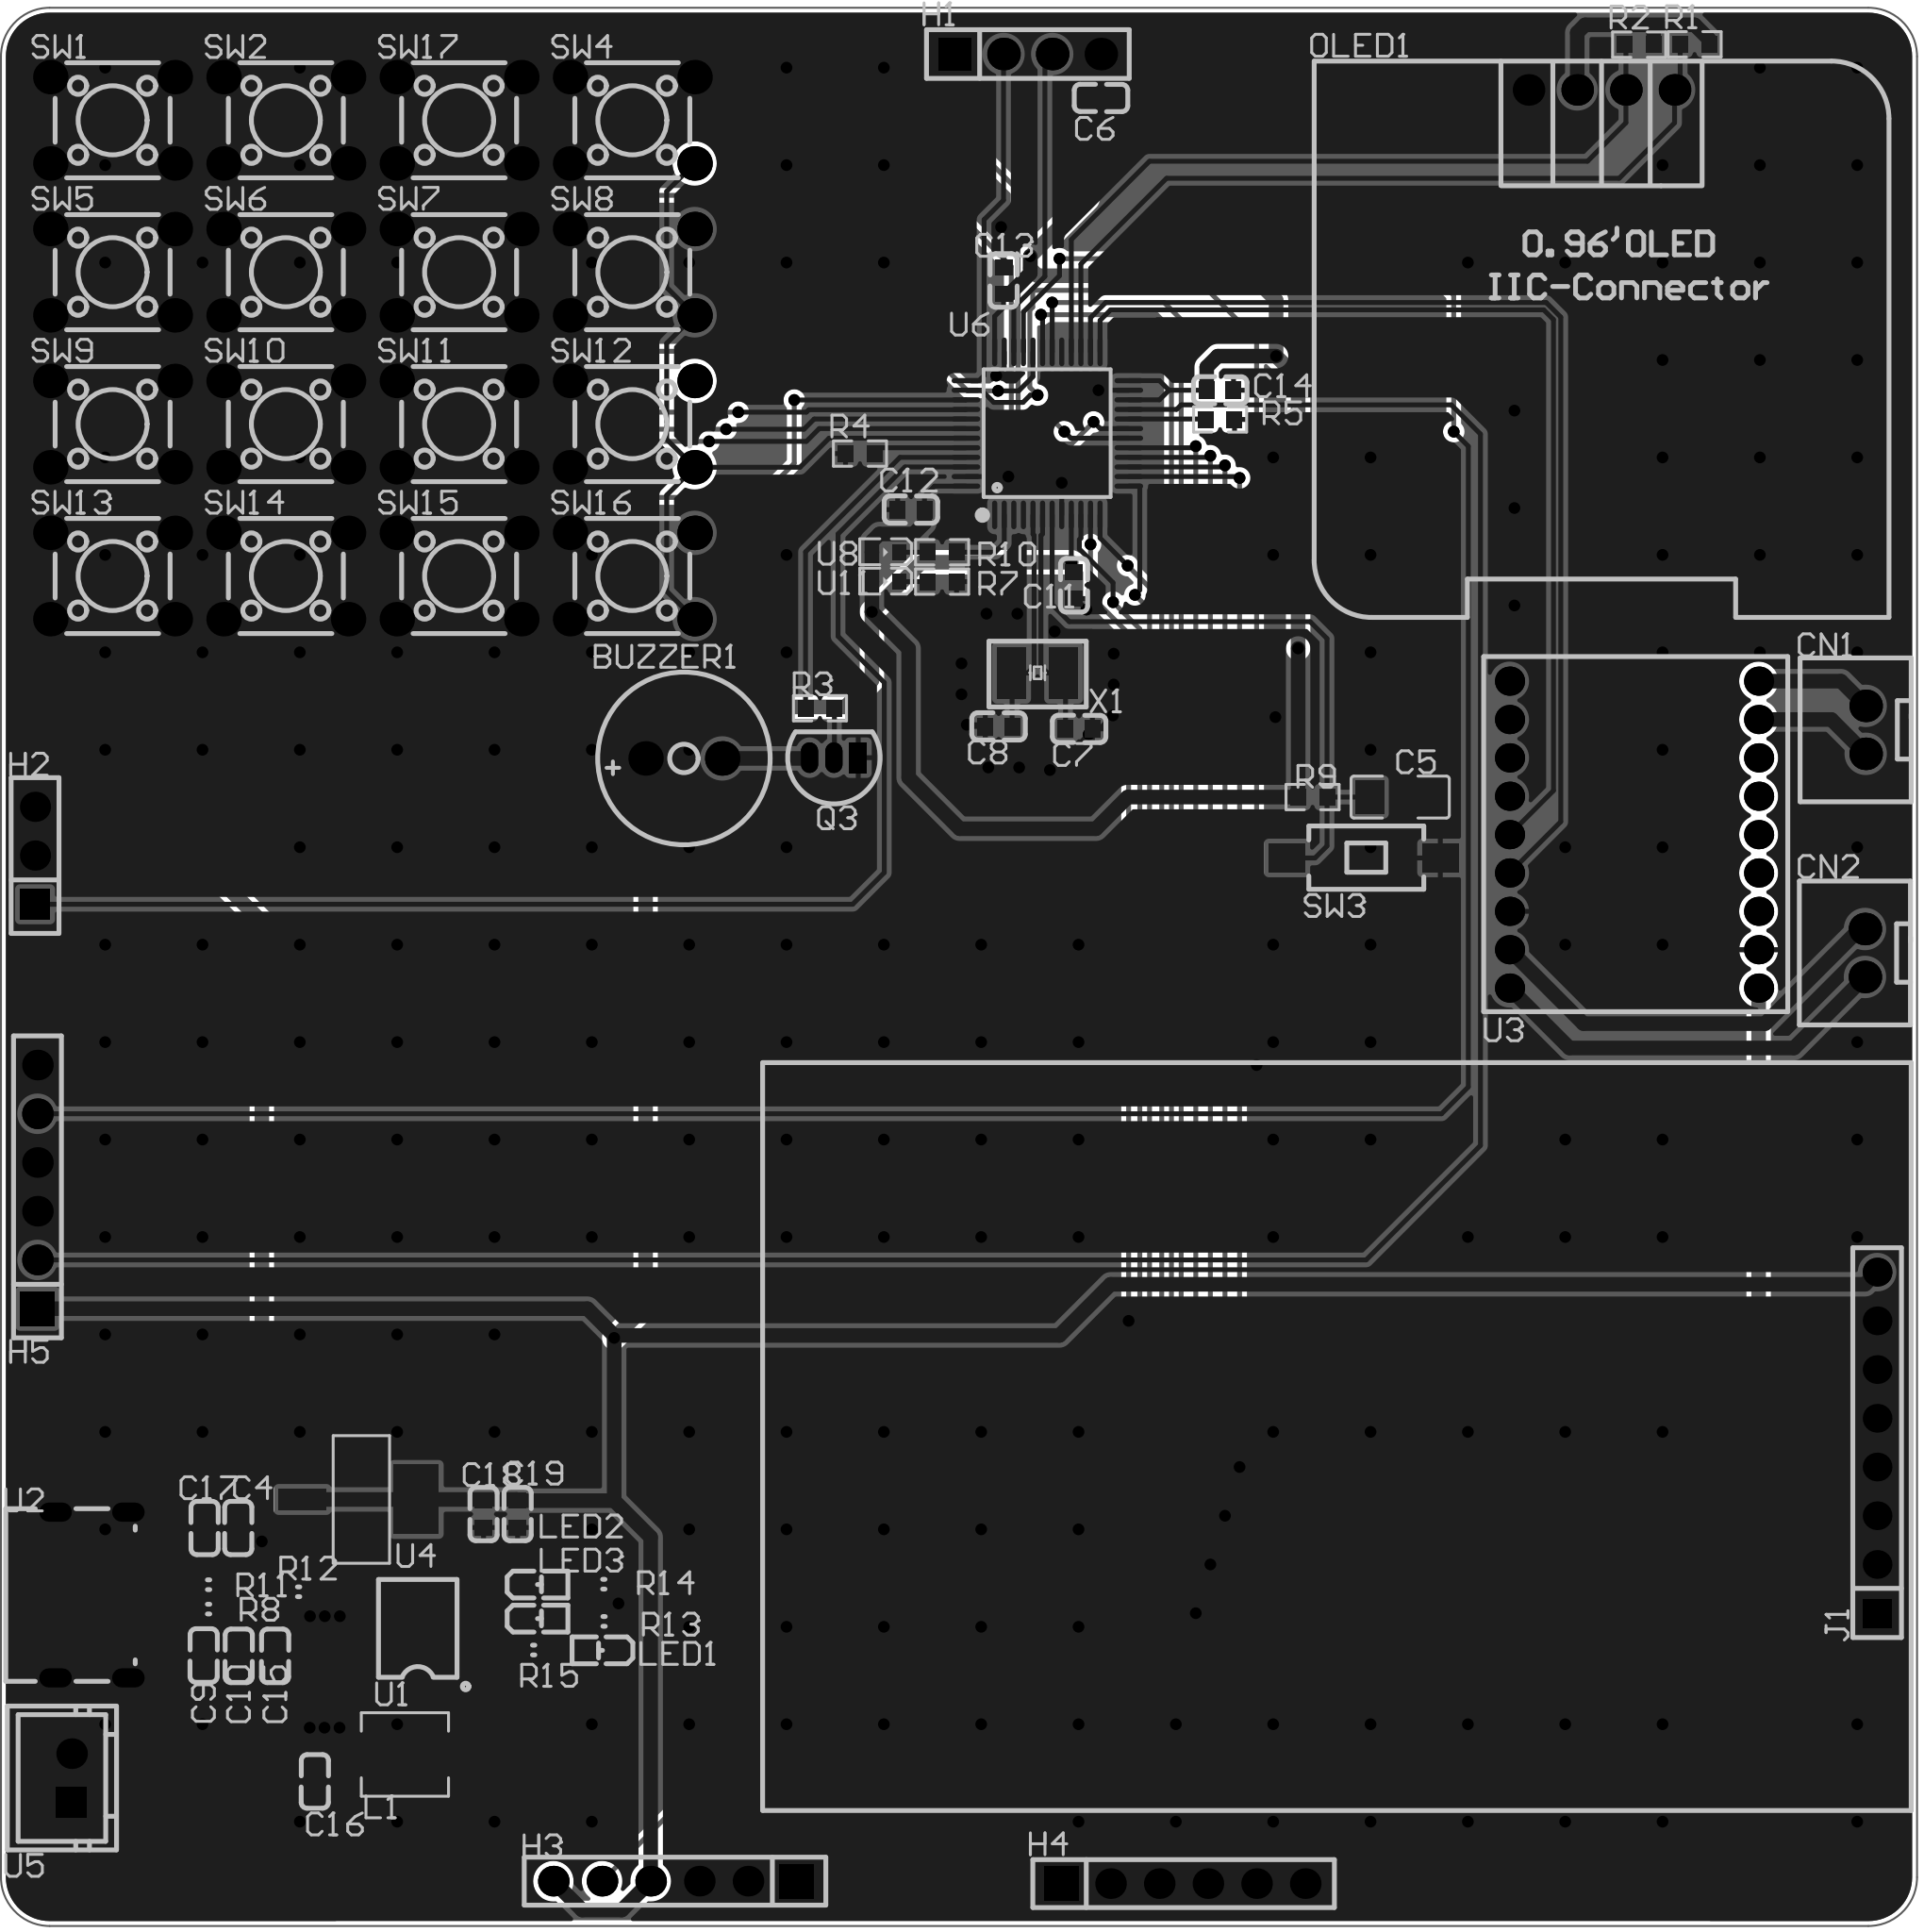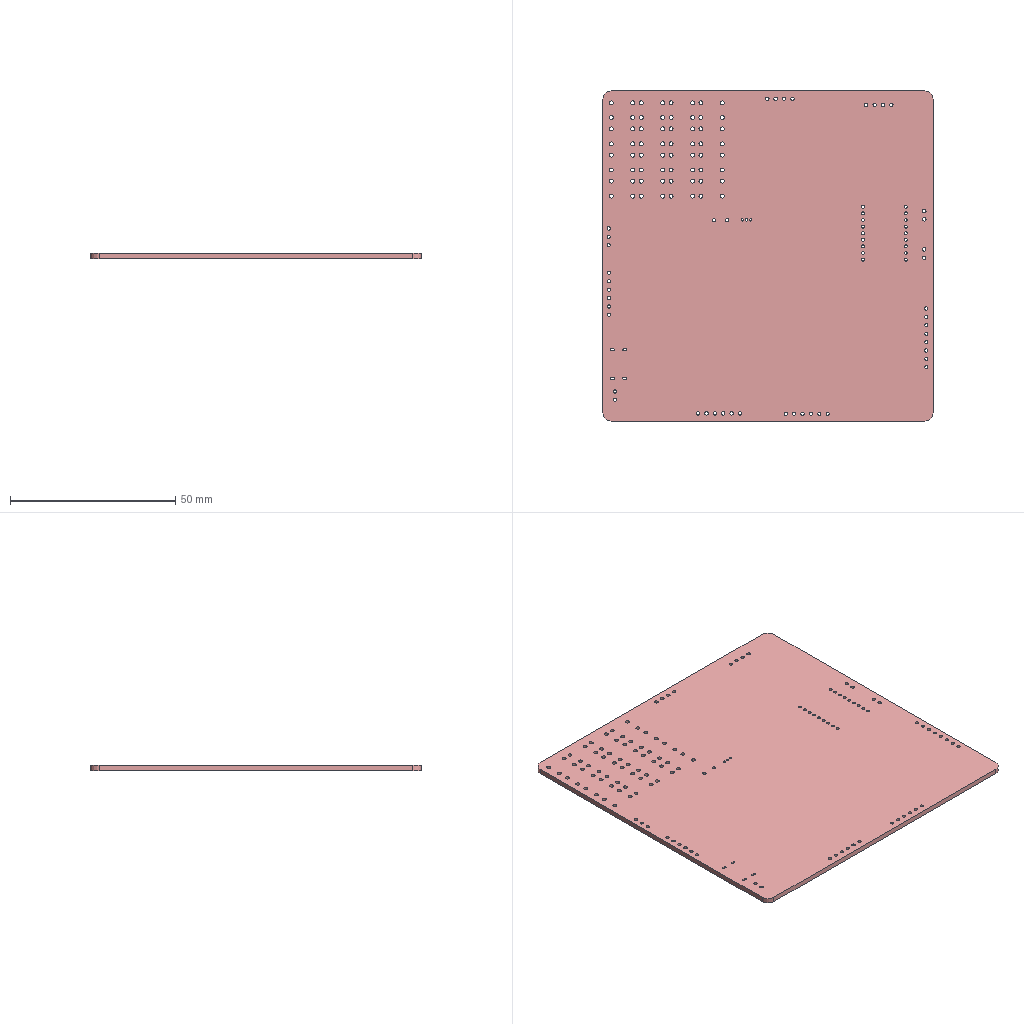Circuit board layout | Altium Designer | box 100 x 100 x 1.6 mm
Layer stack:
# Altium Designer layer stack of  (unit mm; dielectric type: 0 none, 1 core, 2 prepreg, 3 surface material)
index,name,kind,layer,copper_thickness_mm,dielectric_type,dielectric_thickness_mm,dielectric_material,dielectric_constant
0,Top Paste Mask Layer,other,,,,,,
1,Top Silkscreen Layer,other,,,,,,
2,Top Solder Mask Layer,dielectric,,,3,0.01,,3.3
3,Top Layer,copper,Top Layer,0.035,,,,
4,Dielectric1,dielectric,,,3,1.51,FR4,4.5
5,Bottom Layer,copper,Bottom Layer,0.035,,,,
6,Bottom Solder Mask Layer,dielectric,,,3,0.01,,3.3
7,Bottom Silkscreen Layer,other,,,,,,
8,Bottom Paste Mask Layer,other,,,,,,
# drill layer pairs: low layer,high layer
drill_pair,Top Layer,Bottom Layer
Part placement:
Designator,Comment,Layer,Footprint,Center-X(mm),Center-Y(mm),Rotation
BUZZER1,2.7kHz,TopLayer,BUZ-TH_BD9.0-P4.00-D0.6-FD,115.399,144.382,0
C4,10uF,TopLayer,C0603,92.139,104.263,270
C5,100uF,TopLayer,C1206,152.781,142.367,180
C6,100nF,TopLayer,C0603,137.16,178.816,180
C7,20pF,TopLayer,C0603,136.017,145.923,180
C8,20pF,TopLayer,C0603,131.826,146.05,0
C9,22uF,TopLayer,C0603,90.337,97.623,90
C10,22uF,TopLayer,C0603,92.167,97.605,90
C11,100nF,TopLayer,C0603,135.763,153.416,90
C12,100nF,TopLayer,C0603,127.254,157.353,0
C13,100nF,TopLayer,C0603,132.08,169.291,270
C14,100nF,TopLayer,C0603,143.383,163.576,180
C15,22uF,TopLayer,C0603,94.066,97.605,90
C16,22uF,TopLayer,C0603,96.139,91.059,90
C17,100nF,TopLayer,C0603,90.383,104.263,270
C18,10uF,TopLayer,C0603,104.942,104.989,90
C19,100nF,TopLayer,C0603,106.72,104.989,90
CN1,XH2.54*2P_直插,TopLayer,CONN-TH_2P-P2.50-XH2.54-2P,177.077,145.871,270
CN2,XH2.54*2P_直插,TopLayer,CONN-TH_2P-P2.50-XH2.54-2P,177.038,134.239,270
H1,,TopLayer,HDR-TH_4P-P2.54-V-F,133.35,181.102,0
H2,,TopLayer,HDR-TH_3P-P2.54-V-F,81.534,139.319,90
H3,,TopLayer,HDR-TH_6P-P2.54-V-F,114.935,85.852,180
H4,,TopLayer,HDR-TH_6P-P2.54-V-F,141.478,85.725,0
H5,,TopLayer,HDR-TH_6P-P2.54-V-F,81.661,122.047,90
J1,,TopLayer,HDR-TH_8P-P2.54-V-M,177.673,108.712,90
L1,2.2uH,TopLayer,IND-SMD_L4.4-W4.2,100.838,92.456,180
LED1,电池,TopLayer,LED0603_L1.6-W0.8-RD_BLUE,111.033,97.885,180
LED2,放电,TopLayer,LED0603_L1.6-W0.8-RD_BLUE,107.874,101.316,0
LED3,充电,TopLayer,LED0603_L1.6-W0.8-RD_BLUE,107.874,99.538,0
OLED1,,TopLayer,0.96OLED_4P,163.291,179.234,0
Q3,,TopLayer,S8050_TO_92,123.226,144.422,180
R1,5.1K,TopLayer,R0603,168.148,181.61,0
R2,5.1K,TopLayer,R0603,165.252,181.593,0
R4,10kΩ,TopLayer,R0603,124.587,160.274,0
R5,10kΩ,TopLayer,R0603,143.383,162.052,180
R7,510Ω,TopLayer,R0603,128.875,153.599,0
R8,5.1K,TopLayer,R0603-NSK,90.591,100.036,180
R9,1kΩ,TopLayer,R0603,148.209,142.367,180
R10,510Ω,TopLayer,R0603,128.875,155.131,0
R11,5.1K,TopLayer,R0603-NSK,90.591,101.306,180
R12,56K,TopLayer,R0603-NSK,95.29,100.937,180
R13,5.1K,TopLayer,R0603-NSK,111.232,99.394,180
R14,5.1K,TopLayer,R0603-NSK,111.218,101.333,180
R15,5.1K,TopLayer,R0603-NSK,107.557,97.901,180
SW1,KH-6X6X6H-TJ,TopLayer,SW-TH_4P-L6.0-W6.0-P4.50-LS6.5,85.583,177.649,0
SW2,KH-6X6X6H-TJ,TopLayer,SW-TH_4P-L6.0-W6.0-P4.50-LS6.5,94.624,177.649,0
SW3,TS-1101-C-W,TopLayer,SW-SMD_L6.0-W3.3-LS8.0,150.876,139.192,180
SW4,KH-6X6X6H-TJ,TopLayer,SW-TH_4P-L6.0-W6.0-P4.50-LS6.5,112.707,177.649,0
SW5,KH-6X6X6H-TJ,TopLayer,SW-TH_4P-L6.0-W6.0-P4.50-LS6.5,85.583,169.73,0
SW6,KH-6X6X6H-TJ,TopLayer,SW-TH_4P-L6.0-W6.0-P4.50-LS6.5,94.624,169.73,0
SW7,KH-6X6X6H-TJ,TopLayer,SW-TH_4P-L6.0-W6.0-P4.50-LS6.5,103.666,169.73,0
SW8,KH-6X6X6H-TJ,TopLayer,SW-TH_4P-L6.0-W6.0-P4.50-LS6.5,112.707,169.73,0
SW9,KH-6X6X6H-TJ,TopLayer,SW-TH_4P-L6.0-W6.0-P4.50-LS6.5,85.583,161.81,0
SW10,KH-6X6X6H-TJ,TopLayer,SW-TH_4P-L6.0-W6.0-P4.50-LS6.5,94.624,161.81,0
SW11,KH-6X6X6H-TJ,TopLayer,SW-TH_4P-L6.0-W6.0-P4.50-LS6.5,103.666,161.81,0
SW12,KH-6X6X6H-TJ,TopLayer,SW-TH_4P-L6.0-W6.0-P4.50-LS6.5,112.707,161.81,0
SW13,KH-6X6X6H-TJ,TopLayer,SW-TH_4P-L6.0-W6.0-P4.50-LS6.5,85.583,153.892,0
SW14,KH-6X6X6H-TJ,TopLayer,SW-TH_4P-L6.0-W6.0-P4.50-LS6.5,94.624,153.892,0
SW15,KH-6X6X6H-TJ,TopLayer,SW-TH_4P-L6.0-W6.0-P4.50-LS6.5,103.666,153.892,0
SW16,KH-6X6X6H-TJ,TopLayer,SW-TH_4P-L6.0-W6.0-P4.50-LS6.5,112.707,153.892,0
SW17,KH-6X6X6H-TJ,TopLayer,SW-TH_4P-L6.0-W6.0-P4.50-LS6.5,103.666,177.649,0
U1,ETA9742,TopLayer,ESOP-8_L4.9-W3.9-P1.27-LS6.0-BL-EP,101.508,99.03,90
U2,YTC-TC6-268,TopLayer,TYPE-C-SMD_YIYUAN_YTC-TC6-268,84.731,100.77,270
U3,CON2.0MM-PAD-18,TopLayer,CONN-TH_18P-P2.00_C9900078766,164.989,140.41,90
U4,AMS1117-3.3,TopLayer,SOT-223-3_L6.5-W3.4-P2.30-LS7.0-BR,98.465,105.751,180
U6,STM32F103C8T6,TopLayer,LQFP-48_L7.0-W7.0-P0.50-LS9.0-BL,134.367,161.326,0
U8,42-51/GHC-YW2X2K/3T,TopLayer,LED-SMD_L1.6-W0.8-FD_GREEN-1,125.925,155.131,0
U11,42-51/GHC-YW2X2K/3T,TopLayer,LED-SMD_L1.6-W0.8-FD_GREEN-1,125.925,153.599,0
X1,8MHz,TopLayer,CRYSTAL-SMD_L3.2-W2.5_3225-8MHZ,133.858,148.844,180
R3,1K,TopLayer,R0603,122.501,146.998,180
U5,_x001F_XH2.54-2P,TopLayer,CONN-TH_2P-P2.54-V,83.445,91.23,90
Pad and via stacks:
# Altium Designer via and pad stacks of  (unit mm). Each distinct definition once, with the count of objects using it.
# via: kind,start_layer,end_layer,hole_mm,diameter_mm,mode(0 simple;1 top-mid-bottom;2 full stack),diameter_per_layer,count,example_net
# pad: kind,layer,hole_mm,hole_type(0 round;1 square;2 slot),plating,top_size,top_shape(1 round;2 rect;3 octagon;9 rounded rect),mid_size,bottom_size,mode,footprint,size_per_layer,count,example
pad,Multi-Layer,1,0,plated,1.8x1.8,1,1.8x1.8,1.8x1.8,0,BUZ-TH_BD9.0-P4.00-D0.6-FD,,2,BUZZER1.1
pad,Multi-Layer,1.05,0,plated,1.7x1.7,1,1.7x1.7,1.7x1.7,0,CONN-TH_2P-P2.50-XH2.54-2P,,4,CN1.2
pad,Multi-Layer,1.1,0,plated,1.7x1.7,2,1.7x1.7,1.7x1.7,0,HDR-TH_4P-P2.54-V-F,,1,H1.1
pad,Multi-Layer,1.1,0,plated,1.7x1.7,1,1.7x1.7,1.7x1.7,0,HDR-TH_4P-P2.54-V-F,,3,H1.2
pad,Multi-Layer,1.02,0,plated,1.575x1.575,1,1.575x1.575,1.575x1.575,0,HDR-TH_3P-P2.54-V-F,,2,H2.3
pad,Multi-Layer,1.02,0,plated,1.575x1.575,2,1.575x1.575,1.575x1.575,0,HDR-TH_3P-P2.54-V-F,,1,H2.1
pad,Multi-Layer,1.02,0,plated,1.6x1.6,1,1.6x1.6,1.6x1.6,0,HDR-TH_6P-P2.54-V-F,,15,H3.6
pad,Multi-Layer,1.02,0,plated,1.8x1.8,2,1.8x1.8,1.8x1.8,0,HDR-TH_6P-P2.54-V-F,,3,H3.1
pad,Multi-Layer,1,0,plated,1.5x1.5,2,1.5x1.5,1.5x1.5,0,HDR-TH_8P-P2.54-V-M,,1,J1.1
pad,Multi-Layer,1,0,plated,1.5x1.5,1,1.5x1.5,1.5x1.5,0,HDR-TH_8P-P2.54-V-M,,7,J1.2
pad,Multi-Layer,1,0,plated,1.65x1.65,1,1.65x1.65,1.65x1.65,0,0.96OLED_4P,,4,OLED1.4
pad,Multi-Layer,0.701,0,plated,0.8992x1.6,2,0.8992x1.6,0.8992x1.6,0,S8050_TO_92,,1,Q3.1
pad,Multi-Layer,0.701,0,plated,0.8992x1.6,1,0.8992x1.6,0.8992x1.6,0,S8050_TO_92,,2,Q3.2
pad,Multi-Layer,1.2,0,plated,1.8x1.8,1,1.8x1.8,1.8x1.8,0,SW-TH_4P-L6.0-W6.0-P4.50-LS6.5,,64,SW1.1
pad,Multi-Layer,0.6,2,plated,1x1.7,1,1x1.7,1x1.7,0,TYPE-C-SMD_YIYUAN_YTC-TC6-268,,4,U2.3
pad,Multi-Layer,0.9,0,plated,1.524x1.524,1,1.524x1.524,1.524x1.524,0,CONN-TH_18P-P2.00_C9900078766,,18,U3.1
pad,Multi-Layer,1,0,plated,1.6x1.6,1,1.6x1.6,1.6x1.6,0,CONN-TH_2P-P2.54-V,,1,U5.2
pad,Multi-Layer,1,0,plated,1.6x1.6,2,1.6x1.6,1.6x1.6,0,CONN-TH_2P-P2.54-V,,1,U5.1
pad,Top Layer,0,0,plated,0.8x0.9,2,0.8x0.9,0.8x0.9,0,C0603,,30,C4.2
pad,Top Layer,0,0,plated,1.485x1.728,2,1.485x1.728,1.485x1.728,0,C1206,,2,C5.2
pad,Top Layer,0,0,plated,1.4x2.12,2,1.4x2.12,1.4x2.12,0,IND-SMD_L4.4-W4.2,,2,L1.1
pad,Top Layer,0,0,plated,0.8x0.8,2,0.8x0.8,0.8x0.8,0,LED0603_L1.6-W0.8-RD_BLUE,,6,LED1.2
pad,Top Layer,0,0,plated,0.8065x0.864,2,0.8065x0.864,0.8065x0.864,0,R0603,,16,R1.2
pad,Top Layer,0,0,plated,0.8065x0.864,2,0.8065x0.864,0.8065x0.864,0,R0603-NSK,,12,R8.2
pad,Top Layer,0,0,plated,1.9x1.5,2,1.9x1.5,1.9x1.5,0,SW-SMD_L6.0-W3.3-LS8.0,,2,SW3.1
pad,Top Layer,0,0,plated,0.6x1.2,2,0.6x1.2,0.6x1.2,0,ESOP-8_L4.9-W3.9-P1.27-LS6.0-BL-EP,,8,U1.1
pad,Top Layer,0,0,plated,3.5x2.5,2,3.5x2.5,3.5x2.5,0,ESOP-8_L4.9-W3.9-P1.27-LS6.0-BL-EP,,1,U1.9
pad,Top Layer,0,0,plated,0.8x1.6,2,0.8x1.6,0.8x1.6,0,TYPE-C-SMD_YIYUAN_YTC-TC6-268,,2,U2.A12
pad,Top Layer,0,0,plated,0.76x1.6,2,0.76x1.6,0.76x1.6,0,TYPE-C-SMD_YIYUAN_YTC-TC6-268,,2,U2.A9
pad,Top Layer,0,0,plated,0.7x1.6,2,0.7x1.6,0.7x1.6,0,TYPE-C-SMD_YIYUAN_YTC-TC6-268,,2,U2.B5
pad,Top Layer,0,0,plated,2.5x1.1,2,2.5x1.1,2.5x1.1,0,SOT-223-3_L6.5-W3.4-P2.30-LS7.0-BR,,3,U4.1
pad,Top Layer,0,0,plated,2.34x3.6,2,2.34x3.6,2.34x3.6,0,SOT-223-3_L6.5-W3.4-P2.30-LS7.0-BR,,1,U4.4
pad,Top Layer,0,0,plated,0.27x1.5,1,0.27x1.5,0.27x1.5,0,LQFP-48_L7.0-W7.0-P0.50-LS9.0-BL,,24,U6.1
pad,Top Layer,0,0,plated,1.5x0.27,1,1.5x0.27,1.5x0.27,0,LQFP-48_L7.0-W7.0-P0.50-LS9.0-BL,,24,U6.13
pad,Top Layer,0,0,plated,0.8x0.7,2,0.8x0.7,0.8x0.7,0,LED-SMD_L1.6-W0.8-FD_GREEN-1,,4,U8.1
pad,Top Layer,0,0,plated,1.524x2.7,2,1.524x2.7,1.524x2.7,0,CRYSTAL-SMD_L3.2-W2.5_3225-8MHZ,,2,X1.1
via,Top Layer,Bottom Layer,0.3048,0.61,0,,263,MFR_RST
Copper pours:
name,layer,net,type(0 solid;1 hatched;2 none)
Top Layer-GND,Top Layer,GND,0
Bottom Layer-GND,Bottom Layer,GND,0